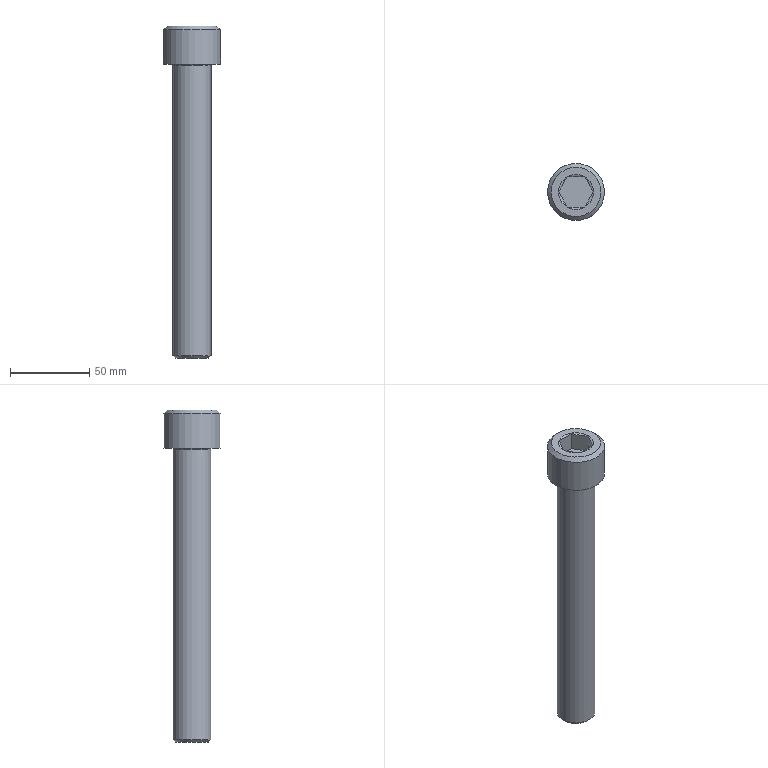Part | STEP file | solid 109 | 1 solid | 21 faces | box 36 x 36 x 209.5 mm | volume 104197 mm3 | plane 10 | sphere 6 | cylinder 2 | cone 2 | torus 1 | commonest cylinder face diameters 24 x1 36 x1